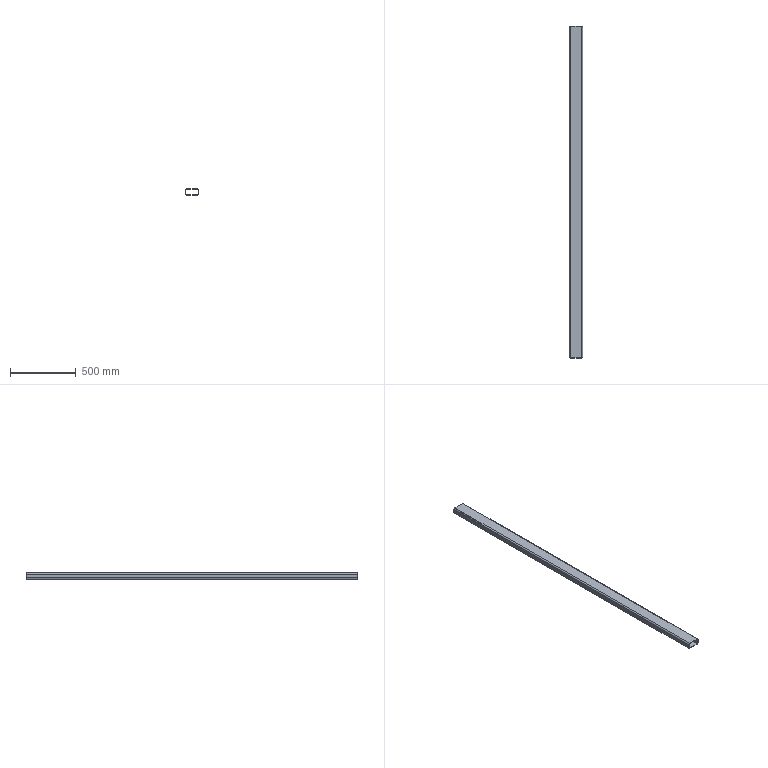Part | SolidWorks | features ExtruThin 1 | 1 solid | 18 faces | box 100 x 2530 x 50 mm | volume 2735087 mm3 | plane 10 | cylinder 8 | commonest cylinder face diameters 12 x4 20 x4
STEP:
#1=CARTESIAN_POINT('',(50.,1265.,-15.));
#2=VERTEX_POINT('',#1);
#3=CARTESIAN_POINT('',(40.,1265.,-25.));
#4=VERTEX_POINT('',#3);
#5=CARTESIAN_POINT('',(40.,1265.,-15.));
#6=DIRECTION('',(0.,1.,0.));
#7=DIRECTION('',(0.,0.,-1.));
#8=AXIS2_PLACEMENT_3D('',#5,#6,#7);
#9=CIRCLE('',#8,10.);
#10=EDGE_CURVE('',#2,#4,#9,.T.);
#11=ORIENTED_EDGE('',*,*,#10,.T.);
#12=CARTESIAN_POINT('',(-40.,1265.,-25.));
#13=VERTEX_POINT('',#12);
#14=CARTESIAN_POINT('',(-40.,1265.,-25.));
#15=DIRECTION('',(-1.,0.,0.));
#16=VECTOR('',#15,1000.);
#17=LINE('',#14,#16);
#18=EDGE_CURVE('',#4,#13,#17,.T.);
#19=ORIENTED_EDGE('',*,*,#18,.T.);
#20=CARTESIAN_POINT('',(-50.,1265.,-15.));
#21=VERTEX_POINT('',#20);
#22=CARTESIAN_POINT('',(-40.,1265.,-15.));
#23=DIRECTION('',(0.,1.,0.));
#24=DIRECTION('',(0.,0.,1.));
#25=AXIS2_PLACEMENT_3D('',#22,#23,#24);
#26=CIRCLE('',#25,10.);
#27=EDGE_CURVE('',#13,#21,#26,.T.);
#28=ORIENTED_EDGE('',*,*,#27,.T.);
#29=CARTESIAN_POINT('',(-50.,1265.,15.));
#30=VERTEX_POINT('',#29);
#31=CARTESIAN_POINT('',(-50.,1265.,-15.));
#32=DIRECTION('',(0.,0.,1.));
#33=VECTOR('',#32,1000.);
#34=LINE('',#31,#33);
#35=EDGE_CURVE('',#21,#30,#34,.T.);
#36=ORIENTED_EDGE('',*,*,#35,.T.);
#37=CARTESIAN_POINT('',(-40.,1265.,25.));
#38=VERTEX_POINT('',#37);
#39=CARTESIAN_POINT('',(-40.,1265.,15.));
#40=DIRECTION('',(0.,1.,0.));
#41=DIRECTION('',(0.,0.,1.));
#42=AXIS2_PLACEMENT_3D('',#39,#40,#41);
#43=CIRCLE('',#42,10.);
#44=EDGE_CURVE('',#30,#38,#43,.T.);
#45=ORIENTED_EDGE('',*,*,#44,.T.);
#46=CARTESIAN_POINT('',(40.,1265.,25.));
#47=VERTEX_POINT('',#46);
#48=CARTESIAN_POINT('',(-40.,1265.,25.));
#49=DIRECTION('',(1.,0.,0.));
#50=VECTOR('',#49,1000.);
#51=LINE('',#48,#50);
#52=EDGE_CURVE('',#38,#47,#51,.T.);
#53=ORIENTED_EDGE('',*,*,#52,.T.);
#54=CARTESIAN_POINT('',(50.,1265.,15.));
#55=VERTEX_POINT('',#54);
#56=CARTESIAN_POINT('',(40.,1265.,15.));
#57=DIRECTION('',(0.,1.,0.));
#58=DIRECTION('',(0.,0.,1.));
#59=AXIS2_PLACEMENT_3D('',#56,#57,#58);
#60=CIRCLE('',#59,10.);
#61=EDGE_CURVE('',#47,#55,#60,.T.);
#62=ORIENTED_EDGE('',*,*,#61,.T.);
#63=CARTESIAN_POINT('',(50.,1265.,-15.));
#64=DIRECTION('',(0.,0.,-1.));
#65=VECTOR('',#64,1000.);
#66=LINE('',#63,#65);
#67=EDGE_CURVE('',#55,#2,#66,.T.);
#68=ORIENTED_EDGE('',*,*,#67,.T.);
#69=EDGE_LOOP('',(#11,#19,#28,#36,#45,#53,#62,#68));
#70=FACE_OUTER_BOUND('',#69,.T.);
#71=CARTESIAN_POINT('',(40.,1265.,-21.));
#72=VERTEX_POINT('',#71);
#73=CARTESIAN_POINT('',(-40.,1265.,-21.));
#74=VERTEX_POINT('',#73);
#75=CARTESIAN_POINT('',(40.,1265.,-21.));
#76=DIRECTION('',(-1.,0.,0.));
#77=VECTOR('',#76,1000.);
#78=LINE('',#75,#77);
#79=EDGE_CURVE('',#72,#74,#78,.T.);
#80=ORIENTED_EDGE('',*,*,#79,.F.);
#81=CARTESIAN_POINT('',(46.,1265.,-15.));
#82=VERTEX_POINT('',#81);
#83=CARTESIAN_POINT('',(40.,1265.,-15.));
#84=DIRECTION('',(0.,1.,0.));
#85=DIRECTION('',(-1.,0.,0.));
#86=AXIS2_PLACEMENT_3D('',#83,#84,#85);
#87=CIRCLE('',#86,6.);
#88=EDGE_CURVE('',#82,#72,#87,.T.);
#89=ORIENTED_EDGE('',*,*,#88,.F.);
#90=CARTESIAN_POINT('',(46.,1265.,15.));
#91=VERTEX_POINT('',#90);
#92=CARTESIAN_POINT('',(46.,1265.,-15.));
#93=DIRECTION('',(0.,0.,-1.));
#94=VECTOR('',#93,1000.);
#95=LINE('',#92,#94);
#96=EDGE_CURVE('',#91,#82,#95,.T.);
#97=ORIENTED_EDGE('',*,*,#96,.F.);
#98=CARTESIAN_POINT('',(40.,1265.,21.));
#99=VERTEX_POINT('',#98);
#100=CARTESIAN_POINT('',(40.,1265.,15.));
#101=DIRECTION('',(0.,1.,0.));
#102=DIRECTION('',(-1.,0.,0.));
#103=AXIS2_PLACEMENT_3D('',#100,#101,#102);
#104=CIRCLE('',#103,6.);
#105=EDGE_CURVE('',#99,#91,#104,.T.);
#106=ORIENTED_EDGE('',*,*,#105,.F.);
#107=CARTESIAN_POINT('',(-40.,1265.,21.));
#108=VERTEX_POINT('',#107);
#109=CARTESIAN_POINT('',(40.,1265.,21.));
#110=DIRECTION('',(1.,0.,0.));
#111=VECTOR('',#110,1000.);
#112=LINE('',#109,#111);
#113=EDGE_CURVE('',#108,#99,#112,.T.);
#114=ORIENTED_EDGE('',*,*,#113,.F.);
#115=CARTESIAN_POINT('',(-46.,1265.,15.));
#116=VERTEX_POINT('',#115);
#117=CARTESIAN_POINT('',(-40.,1265.,15.));
#118=DIRECTION('',(0.,1.,0.));
#119=DIRECTION('',(-1.,0.,0.));
#120=AXIS2_PLACEMENT_3D('',#117,#118,#119);
#121=CIRCLE('',#120,6.);
#122=EDGE_CURVE('',#116,#108,#121,.T.);
#123=ORIENTED_EDGE('',*,*,#122,.F.);
#124=CARTESIAN_POINT('',(-46.,1265.,-15.));
#125=VERTEX_POINT('',#124);
#126=CARTESIAN_POINT('',(-46.,1265.,-15.));
#127=DIRECTION('',(0.,0.,1.));
#128=VECTOR('',#127,1000.);
#129=LINE('',#126,#128);
#130=EDGE_CURVE('',#125,#116,#129,.T.);
#131=ORIENTED_EDGE('',*,*,#130,.F.);
#132=CARTESIAN_POINT('',(-40.,1265.,-15.));
#133=DIRECTION('',(0.,1.,0.));
#134=DIRECTION('',(-1.,0.,0.));
#135=AXIS2_PLACEMENT_3D('',#132,#133,#134);
#136=CIRCLE('',#135,6.);
#137=EDGE_CURVE('',#74,#125,#136,.T.);
#138=ORIENTED_EDGE('',*,*,#137,.F.);
#139=EDGE_LOOP('',(#80,#89,#97,#106,#114,#123,#131,#138));
#140=FACE_BOUND('',#139,.T.);
#141=CARTESIAN_POINT('',(40.,1265.,-15.));
#142=DIRECTION('',(0.,1.,0.));
#143=DIRECTION('',(0.,0.,1.));
#144=AXIS2_PLACEMENT_3D('',#141,#142,#143);
#145=PLANE('',#144);
#146=ADVANCED_FACE('',(#70,#140),#145,.T.);
#147=CARTESIAN_POINT('',(50.,-1265.,-15.));
#148=VERTEX_POINT('',#147);
#149=CARTESIAN_POINT('',(40.,-1265.,-25.));
#150=VERTEX_POINT('',#149);
#151=CARTESIAN_POINT('',(40.,-1265.,-15.));
#152=DIRECTION('',(0.,1.,0.));
#153=DIRECTION('',(0.,0.,-1.));
#154=AXIS2_PLACEMENT_3D('',#151,#152,#153);
#155=CIRCLE('',#154,10.);
#156=EDGE_CURVE('',#148,#150,#155,.T.);
#157=ORIENTED_EDGE('',*,*,#156,.F.);
#158=CARTESIAN_POINT('',(50.,-1265.,15.));
#159=VERTEX_POINT('',#158);
#160=CARTESIAN_POINT('',(50.,-1265.,-15.));
#161=DIRECTION('',(0.,0.,-1.));
#162=VECTOR('',#161,1000.);
#163=LINE('',#160,#162);
#164=EDGE_CURVE('',#159,#148,#163,.T.);
#165=ORIENTED_EDGE('',*,*,#164,.F.);
#166=CARTESIAN_POINT('',(40.,-1265.,25.));
#167=VERTEX_POINT('',#166);
#168=CARTESIAN_POINT('',(40.,-1265.,15.));
#169=DIRECTION('',(0.,1.,0.));
#170=DIRECTION('',(0.,0.,1.));
#171=AXIS2_PLACEMENT_3D('',#168,#169,#170);
#172=CIRCLE('',#171,10.);
#173=EDGE_CURVE('',#167,#159,#172,.T.);
#174=ORIENTED_EDGE('',*,*,#173,.F.);
#175=CARTESIAN_POINT('',(-40.,-1265.,25.));
#176=VERTEX_POINT('',#175);
#177=CARTESIAN_POINT('',(-40.,-1265.,25.));
#178=DIRECTION('',(1.,0.,0.));
#179=VECTOR('',#178,1000.);
#180=LINE('',#177,#179);
#181=EDGE_CURVE('',#176,#167,#180,.T.);
#182=ORIENTED_EDGE('',*,*,#181,.F.);
#183=CARTESIAN_POINT('',(-50.,-1265.,15.));
#184=VERTEX_POINT('',#183);
#185=CARTESIAN_POINT('',(-40.,-1265.,15.));
#186=DIRECTION('',(0.,1.,0.));
#187=DIRECTION('',(0.,0.,1.));
#188=AXIS2_PLACEMENT_3D('',#185,#186,#187);
#189=CIRCLE('',#188,10.);
#190=EDGE_CURVE('',#184,#176,#189,.T.);
#191=ORIENTED_EDGE('',*,*,#190,.F.);
#192=CARTESIAN_POINT('',(-50.,-1265.,-15.));
#193=VERTEX_POINT('',#192);
#194=CARTESIAN_POINT('',(-50.,-1265.,-15.));
#195=DIRECTION('',(0.,0.,1.));
#196=VECTOR('',#195,1000.);
#197=LINE('',#194,#196);
#198=EDGE_CURVE('',#193,#184,#197,.T.);
#199=ORIENTED_EDGE('',*,*,#198,.F.);
#200=CARTESIAN_POINT('',(-40.,-1265.,-25.));
#201=VERTEX_POINT('',#200);
#202=CARTESIAN_POINT('',(-40.,-1265.,-15.));
#203=DIRECTION('',(0.,1.,0.));
#204=DIRECTION('',(0.,0.,1.));
#205=AXIS2_PLACEMENT_3D('',#202,#203,#204);
#206=CIRCLE('',#205,10.);
#207=EDGE_CURVE('',#201,#193,#206,.T.);
#208=ORIENTED_EDGE('',*,*,#207,.F.);
#209=CARTESIAN_POINT('',(-40.,-1265.,-25.));
#210=DIRECTION('',(-1.,0.,0.));
#211=VECTOR('',#210,1000.);
#212=LINE('',#209,#211);
#213=EDGE_CURVE('',#150,#201,#212,.T.);
#214=ORIENTED_EDGE('',*,*,#213,.F.);
#215=EDGE_LOOP('',(#157,#165,#174,#182,#191,#199,#208,#214));
#216=FACE_OUTER_BOUND('',#215,.T.);
#217=CARTESIAN_POINT('',(46.,-1265.,-15.));
#218=VERTEX_POINT('',#217);
#219=CARTESIAN_POINT('',(40.,-1265.,-21.));
#220=VERTEX_POINT('',#219);
#221=CARTESIAN_POINT('',(40.,-1265.,-15.));
#222=DIRECTION('',(0.,1.,0.));
#223=DIRECTION('',(-1.,0.,0.));
#224=AXIS2_PLACEMENT_3D('',#221,#222,#223);
#225=CIRCLE('',#224,6.);
#226=EDGE_CURVE('',#218,#220,#225,.T.);
#227=ORIENTED_EDGE('',*,*,#226,.T.);
#228=CARTESIAN_POINT('',(-40.,-1265.,-21.));
#229=VERTEX_POINT('',#228);
#230=CARTESIAN_POINT('',(40.,-1265.,-21.));
#231=DIRECTION('',(-1.,0.,0.));
#232=VECTOR('',#231,1000.);
#233=LINE('',#230,#232);
#234=EDGE_CURVE('',#220,#229,#233,.T.);
#235=ORIENTED_EDGE('',*,*,#234,.T.);
#236=CARTESIAN_POINT('',(-46.,-1265.,-15.));
#237=VERTEX_POINT('',#236);
#238=CARTESIAN_POINT('',(-40.,-1265.,-15.));
#239=DIRECTION('',(0.,1.,0.));
#240=DIRECTION('',(-1.,0.,0.));
#241=AXIS2_PLACEMENT_3D('',#238,#239,#240);
#242=CIRCLE('',#241,6.);
#243=EDGE_CURVE('',#229,#237,#242,.T.);
#244=ORIENTED_EDGE('',*,*,#243,.T.);
#245=CARTESIAN_POINT('',(-46.,-1265.,15.));
#246=VERTEX_POINT('',#245);
#247=CARTESIAN_POINT('',(-46.,-1265.,-15.));
#248=DIRECTION('',(0.,0.,1.));
#249=VECTOR('',#248,1000.);
#250=LINE('',#247,#249);
#251=EDGE_CURVE('',#237,#246,#250,.T.);
#252=ORIENTED_EDGE('',*,*,#251,.T.);
#253=CARTESIAN_POINT('',(-40.,-1265.,21.));
#254=VERTEX_POINT('',#253);
#255=CARTESIAN_POINT('',(-40.,-1265.,15.));
#256=DIRECTION('',(0.,1.,0.));
#257=DIRECTION('',(-1.,0.,0.));
#258=AXIS2_PLACEMENT_3D('',#255,#256,#257);
#259=CIRCLE('',#258,6.);
#260=EDGE_CURVE('',#246,#254,#259,.T.);
#261=ORIENTED_EDGE('',*,*,#260,.T.);
#262=CARTESIAN_POINT('',(40.,-1265.,21.));
#263=VERTEX_POINT('',#262);
#264=CARTESIAN_POINT('',(40.,-1265.,21.));
#265=DIRECTION('',(1.,0.,0.));
#266=VECTOR('',#265,1000.);
#267=LINE('',#264,#266);
#268=EDGE_CURVE('',#254,#263,#267,.T.);
#269=ORIENTED_EDGE('',*,*,#268,.T.);
#270=CARTESIAN_POINT('',(46.,-1265.,15.));
#271=VERTEX_POINT('',#270);
#272=CARTESIAN_POINT('',(40.,-1265.,15.));
#273=DIRECTION('',(0.,1.,0.));
#274=DIRECTION('',(-1.,0.,0.));
#275=AXIS2_PLACEMENT_3D('',#272,#273,#274);
#276=CIRCLE('',#275,6.);
#277=EDGE_CURVE('',#263,#271,#276,.T.);
#278=ORIENTED_EDGE('',*,*,#277,.T.);
#279=CARTESIAN_POINT('',(46.,-1265.,-15.));
#280=DIRECTION('',(0.,0.,-1.));
#281=VECTOR('',#280,1000.);
#282=LINE('',#279,#281);
#283=EDGE_CURVE('',#271,#218,#282,.T.);
#284=ORIENTED_EDGE('',*,*,#283,.T.);
#285=EDGE_LOOP('',(#227,#235,#244,#252,#261,#269,#278,#284));
#286=FACE_BOUND('',#285,.T.);
#287=CARTESIAN_POINT('',(40.,-1265.,-15.));
#288=DIRECTION('',(0.,1.,0.));
#289=DIRECTION('',(0.,0.,1.));
#290=AXIS2_PLACEMENT_3D('',#287,#288,#289);
#291=PLANE('',#290);
#292=ADVANCED_FACE('',(#216,#286),#291,.F.);
#293=ORIENTED_EDGE('',*,*,#156,.T.);
#294=CARTESIAN_POINT('',(40.,1265.,-25.));
#295=DIRECTION('',(0.,-1.,0.));
#296=VECTOR('',#295,1000.);
#297=LINE('',#294,#296);
#298=EDGE_CURVE('',#4,#150,#297,.T.);
#299=ORIENTED_EDGE('',*,*,#298,.F.);
#300=ORIENTED_EDGE('',*,*,#10,.F.);
#301=CARTESIAN_POINT('',(50.,1265.,-15.));
#302=DIRECTION('',(0.,-1.,0.));
#303=VECTOR('',#302,1000.);
#304=LINE('',#301,#303);
#305=EDGE_CURVE('',#2,#148,#304,.T.);
#306=ORIENTED_EDGE('',*,*,#305,.T.);
#307=EDGE_LOOP('',(#293,#299,#300,#306));
#308=FACE_OUTER_BOUND('',#307,.T.);
#309=CARTESIAN_POINT('',(40.,1265.,-15.));
#310=DIRECTION('',(0.,-1.,0.));
#311=DIRECTION('',(0.,0.,-1.));
#312=AXIS2_PLACEMENT_3D('',#309,#310,#311);
#313=CYLINDRICAL_SURFACE('',#312,10.);
#314=ADVANCED_FACE('',(#308),#313,.T.);
#315=ORIENTED_EDGE('',*,*,#213,.T.);
#316=CARTESIAN_POINT('',(-40.,1265.,-25.));
#317=DIRECTION('',(0.,-1.,0.));
#318=VECTOR('',#317,1000.);
#319=LINE('',#316,#318);
#320=EDGE_CURVE('',#13,#201,#319,.T.);
#321=ORIENTED_EDGE('',*,*,#320,.F.);
#322=ORIENTED_EDGE('',*,*,#18,.F.);
#323=ORIENTED_EDGE('',*,*,#298,.T.);
#324=EDGE_LOOP('',(#315,#321,#322,#323));
#325=FACE_OUTER_BOUND('',#324,.T.);
#326=CARTESIAN_POINT('',(-40.,1265.,-25.));
#327=DIRECTION('',(0.,0.,1.));
#328=DIRECTION('',(1.,0.,0.));
#329=AXIS2_PLACEMENT_3D('',#326,#327,#328);
#330=PLANE('',#329);
#331=ADVANCED_FACE('',(#325),#330,.F.);
#332=ORIENTED_EDGE('',*,*,#207,.T.);
#333=CARTESIAN_POINT('',(-50.,1265.,-15.));
#334=DIRECTION('',(0.,-1.,0.));
#335=VECTOR('',#334,1000.);
#336=LINE('',#333,#335);
#337=EDGE_CURVE('',#21,#193,#336,.T.);
#338=ORIENTED_EDGE('',*,*,#337,.F.);
#339=ORIENTED_EDGE('',*,*,#27,.F.);
#340=ORIENTED_EDGE('',*,*,#320,.T.);
#341=EDGE_LOOP('',(#332,#338,#339,#340));
#342=FACE_OUTER_BOUND('',#341,.T.);
#343=CARTESIAN_POINT('',(-40.,1265.,-15.));
#344=DIRECTION('',(0.,-1.,0.));
#345=DIRECTION('',(0.,0.,-1.));
#346=AXIS2_PLACEMENT_3D('',#343,#344,#345);
#347=CYLINDRICAL_SURFACE('',#346,10.);
#348=ADVANCED_FACE('',(#342),#347,.T.);
#349=ORIENTED_EDGE('',*,*,#198,.T.);
#350=CARTESIAN_POINT('',(-50.,1265.,15.));
#351=DIRECTION('',(0.,-1.,0.));
#352=VECTOR('',#351,1000.);
#353=LINE('',#350,#352);
#354=EDGE_CURVE('',#30,#184,#353,.T.);
#355=ORIENTED_EDGE('',*,*,#354,.F.);
#356=ORIENTED_EDGE('',*,*,#35,.F.);
#357=ORIENTED_EDGE('',*,*,#337,.T.);
#358=EDGE_LOOP('',(#349,#355,#356,#357));
#359=FACE_OUTER_BOUND('',#358,.T.);
#360=CARTESIAN_POINT('',(-50.,1265.,-15.));
#361=DIRECTION('',(1.,0.,0.));
#362=DIRECTION('',(0.,0.,-1.));
#363=AXIS2_PLACEMENT_3D('',#360,#361,#362);
#364=PLANE('',#363);
#365=ADVANCED_FACE('',(#359),#364,.F.);
#366=ORIENTED_EDGE('',*,*,#190,.T.);
#367=CARTESIAN_POINT('',(-40.,1265.,25.));
#368=DIRECTION('',(0.,-1.,0.));
#369=VECTOR('',#368,1000.);
#370=LINE('',#367,#369);
#371=EDGE_CURVE('',#38,#176,#370,.T.);
#372=ORIENTED_EDGE('',*,*,#371,.F.);
#373=ORIENTED_EDGE('',*,*,#44,.F.);
#374=ORIENTED_EDGE('',*,*,#354,.T.);
#375=EDGE_LOOP('',(#366,#372,#373,#374));
#376=FACE_OUTER_BOUND('',#375,.T.);
#377=CARTESIAN_POINT('',(-40.,1265.,15.));
#378=DIRECTION('',(0.,-1.,0.));
#379=DIRECTION('',(0.,0.,-1.));
#380=AXIS2_PLACEMENT_3D('',#377,#378,#379);
#381=CYLINDRICAL_SURFACE('',#380,10.);
#382=ADVANCED_FACE('',(#376),#381,.T.);
#383=ORIENTED_EDGE('',*,*,#181,.T.);
#384=CARTESIAN_POINT('',(40.,1265.,25.));
#385=DIRECTION('',(0.,-1.,0.));
#386=VECTOR('',#385,1000.);
#387=LINE('',#384,#386);
#388=EDGE_CURVE('',#47,#167,#387,.T.);
#389=ORIENTED_EDGE('',*,*,#388,.F.);
#390=ORIENTED_EDGE('',*,*,#52,.F.);
#391=ORIENTED_EDGE('',*,*,#371,.T.);
#392=EDGE_LOOP('',(#383,#389,#390,#391));
#393=FACE_OUTER_BOUND('',#392,.T.);
#394=CARTESIAN_POINT('',(-40.,1265.,25.));
#395=DIRECTION('',(0.,0.,-1.));
#396=DIRECTION('',(-1.,0.,0.));
#397=AXIS2_PLACEMENT_3D('',#394,#395,#396);
#398=PLANE('',#397);
#399=ADVANCED_FACE('',(#393),#398,.F.);
#400=ORIENTED_EDGE('',*,*,#173,.T.);
#401=CARTESIAN_POINT('',(50.,1265.,15.));
#402=DIRECTION('',(0.,-1.,0.));
#403=VECTOR('',#402,1000.);
#404=LINE('',#401,#403);
#405=EDGE_CURVE('',#55,#159,#404,.T.);
#406=ORIENTED_EDGE('',*,*,#405,.F.);
#407=ORIENTED_EDGE('',*,*,#61,.F.);
#408=ORIENTED_EDGE('',*,*,#388,.T.);
#409=EDGE_LOOP('',(#400,#406,#407,#408));
#410=FACE_OUTER_BOUND('',#409,.T.);
#411=CARTESIAN_POINT('',(40.,1265.,15.));
#412=DIRECTION('',(0.,-1.,0.));
#413=DIRECTION('',(0.,0.,-1.));
#414=AXIS2_PLACEMENT_3D('',#411,#412,#413);
#415=CYLINDRICAL_SURFACE('',#414,10.);
#416=ADVANCED_FACE('',(#410),#415,.T.);
#417=ORIENTED_EDGE('',*,*,#164,.T.);
#418=ORIENTED_EDGE('',*,*,#305,.F.);
#419=ORIENTED_EDGE('',*,*,#67,.F.);
#420=ORIENTED_EDGE('',*,*,#405,.T.);
#421=EDGE_LOOP('',(#417,#418,#419,#420));
#422=FACE_OUTER_BOUND('',#421,.T.);
#423=CARTESIAN_POINT('',(50.,1265.,-15.));
#424=DIRECTION('',(-1.,0.,0.));
#425=DIRECTION('',(0.,0.,1.));
#426=AXIS2_PLACEMENT_3D('',#423,#424,#425);
#427=PLANE('',#426);
#428=ADVANCED_FACE('',(#422),#427,.F.);
#429=ORIENTED_EDGE('',*,*,#226,.F.);
#430=CARTESIAN_POINT('',(46.,1265.,-15.));
#431=DIRECTION('',(0.,-1.,0.));
#432=VECTOR('',#431,1000.);
#433=LINE('',#430,#432);
#434=EDGE_CURVE('',#82,#218,#433,.T.);
#435=ORIENTED_EDGE('',*,*,#434,.F.);
#436=ORIENTED_EDGE('',*,*,#88,.T.);
#437=CARTESIAN_POINT('',(40.,1265.,-21.));
#438=DIRECTION('',(0.,-1.,0.));
#439=VECTOR('',#438,1000.);
#440=LINE('',#437,#439);
#441=EDGE_CURVE('',#72,#220,#440,.T.);
#442=ORIENTED_EDGE('',*,*,#441,.T.);
#443=EDGE_LOOP('',(#429,#435,#436,#442));
#444=FACE_OUTER_BOUND('',#443,.T.);
#445=CARTESIAN_POINT('',(40.,1265.,-15.));
#446=DIRECTION('',(0.,-1.,0.));
#447=DIRECTION('',(0.,0.,-1.));
#448=AXIS2_PLACEMENT_3D('',#445,#446,#447);
#449=CYLINDRICAL_SURFACE('',#448,6.);
#450=ADVANCED_FACE('',(#444),#449,.F.);
#451=ORIENTED_EDGE('',*,*,#234,.F.);
#452=ORIENTED_EDGE('',*,*,#441,.F.);
#453=ORIENTED_EDGE('',*,*,#79,.T.);
#454=CARTESIAN_POINT('',(-40.,1265.,-21.));
#455=DIRECTION('',(0.,-1.,0.));
#456=VECTOR('',#455,1000.);
#457=LINE('',#454,#456);
#458=EDGE_CURVE('',#74,#229,#457,.T.);
#459=ORIENTED_EDGE('',*,*,#458,.T.);
#460=EDGE_LOOP('',(#451,#452,#453,#459));
#461=FACE_OUTER_BOUND('',#460,.T.);
#462=CARTESIAN_POINT('',(40.,1265.,-21.));
#463=DIRECTION('',(0.,0.,1.));
#464=DIRECTION('',(1.,0.,0.));
#465=AXIS2_PLACEMENT_3D('',#462,#463,#464);
#466=PLANE('',#465);
#467=ADVANCED_FACE('',(#461),#466,.T.);
#468=ORIENTED_EDGE('',*,*,#243,.F.);
#469=ORIENTED_EDGE('',*,*,#458,.F.);
#470=ORIENTED_EDGE('',*,*,#137,.T.);
#471=CARTESIAN_POINT('',(-46.,1265.,-15.));
#472=DIRECTION('',(0.,-1.,0.));
#473=VECTOR('',#472,1000.);
#474=LINE('',#471,#473);
#475=EDGE_CURVE('',#125,#237,#474,.T.);
#476=ORIENTED_EDGE('',*,*,#475,.T.);
#477=EDGE_LOOP('',(#468,#469,#470,#476));
#478=FACE_OUTER_BOUND('',#477,.T.);
#479=CARTESIAN_POINT('',(-40.,1265.,-15.));
#480=DIRECTION('',(0.,-1.,0.));
#481=DIRECTION('',(0.,0.,-1.));
#482=AXIS2_PLACEMENT_3D('',#479,#480,#481);
#483=CYLINDRICAL_SURFACE('',#482,6.);
#484=ADVANCED_FACE('',(#478),#483,.F.);
#485=ORIENTED_EDGE('',*,*,#251,.F.);
#486=ORIENTED_EDGE('',*,*,#475,.F.);
#487=ORIENTED_EDGE('',*,*,#130,.T.);
#488=CARTESIAN_POINT('',(-46.,1265.,15.));
#489=DIRECTION('',(0.,-1.,0.));
#490=VECTOR('',#489,1000.);
#491=LINE('',#488,#490);
#492=EDGE_CURVE('',#116,#246,#491,.T.);
#493=ORIENTED_EDGE('',*,*,#492,.T.);
#494=EDGE_LOOP('',(#485,#486,#487,#493));
#495=FACE_OUTER_BOUND('',#494,.T.);
#496=CARTESIAN_POINT('',(-46.,1265.,-15.));
#497=DIRECTION('',(1.,0.,0.));
#498=DIRECTION('',(0.,0.,-1.));
#499=AXIS2_PLACEMENT_3D('',#496,#497,#498);
#500=PLANE('',#499);
#501=ADVANCED_FACE('',(#495),#500,.T.);
#502=ORIENTED_EDGE('',*,*,#260,.F.);
#503=ORIENTED_EDGE('',*,*,#492,.F.);
#504=ORIENTED_EDGE('',*,*,#122,.T.);
#505=CARTESIAN_POINT('',(-40.,1265.,21.));
#506=DIRECTION('',(0.,-1.,0.));
#507=VECTOR('',#506,1000.);
#508=LINE('',#505,#507);
#509=EDGE_CURVE('',#108,#254,#508,.T.);
#510=ORIENTED_EDGE('',*,*,#509,.T.);
#511=EDGE_LOOP('',(#502,#503,#504,#510));
#512=FACE_OUTER_BOUND('',#511,.T.);
#513=CARTESIAN_POINT('',(-40.,1265.,15.));
#514=DIRECTION('',(0.,-1.,0.));
#515=DIRECTION('',(0.,0.,-1.));
#516=AXIS2_PLACEMENT_3D('',#513,#514,#515);
#517=CYLINDRICAL_SURFACE('',#516,6.);
#518=ADVANCED_FACE('',(#512),#517,.F.);
#519=ORIENTED_EDGE('',*,*,#268,.F.);
#520=ORIENTED_EDGE('',*,*,#509,.F.);
#521=ORIENTED_EDGE('',*,*,#113,.T.);
#522=CARTESIAN_POINT('',(40.,1265.,21.));
#523=DIRECTION('',(0.,-1.,0.));
#524=VECTOR('',#523,1000.);
#525=LINE('',#522,#524);
#526=EDGE_CURVE('',#99,#263,#525,.T.);
#527=ORIENTED_EDGE('',*,*,#526,.T.);
#528=EDGE_LOOP('',(#519,#520,#521,#527));
#529=FACE_OUTER_BOUND('',#528,.T.);
#530=CARTESIAN_POINT('',(40.,1265.,21.));
#531=DIRECTION('',(0.,0.,-1.));
#532=DIRECTION('',(-1.,0.,0.));
#533=AXIS2_PLACEMENT_3D('',#530,#531,#532);
#534=PLANE('',#533);
#535=ADVANCED_FACE('',(#529),#534,.T.);
#536=ORIENTED_EDGE('',*,*,#277,.F.);
#537=ORIENTED_EDGE('',*,*,#526,.F.);
#538=ORIENTED_EDGE('',*,*,#105,.T.);
#539=CARTESIAN_POINT('',(46.,1265.,15.));
#540=DIRECTION('',(0.,-1.,0.));
#541=VECTOR('',#540,1000.);
#542=LINE('',#539,#541);
#543=EDGE_CURVE('',#91,#271,#542,.T.);
#544=ORIENTED_EDGE('',*,*,#543,.T.);
#545=EDGE_LOOP('',(#536,#537,#538,#544));
#546=FACE_OUTER_BOUND('',#545,.T.);
#547=CARTESIAN_POINT('',(40.,1265.,15.));
#548=DIRECTION('',(0.,-1.,0.));
#549=DIRECTION('',(0.,0.,-1.));
#550=AXIS2_PLACEMENT_3D('',#547,#548,#549);
#551=CYLINDRICAL_SURFACE('',#550,6.);
#552=ADVANCED_FACE('',(#546),#551,.F.);
#553=ORIENTED_EDGE('',*,*,#283,.F.);
#554=ORIENTED_EDGE('',*,*,#543,.F.);
#555=ORIENTED_EDGE('',*,*,#96,.T.);
#556=ORIENTED_EDGE('',*,*,#434,.T.);
#557=EDGE_LOOP('',(#553,#554,#555,#556));
#558=FACE_OUTER_BOUND('',#557,.T.);
#559=CARTESIAN_POINT('',(46.,1265.,-15.));
#560=DIRECTION('',(-1.,0.,0.));
#561=DIRECTION('',(0.,0.,1.));
#562=AXIS2_PLACEMENT_3D('',#559,#560,#561);
#563=PLANE('',#562);
#564=ADVANCED_FACE('',(#558),#563,.T.);
#565=CLOSED_SHELL('',(#146,#292,#314,#331,#348,#365,#382,#399,#416,#428,#450,#467,#484,#501,#518,#535,#552,#564));
#566=MANIFOLD_SOLID_BREP('',#565);
#567=CARTESIAN_POINT('',(0.,0.,0.));
#568=DIRECTION('',(0.,0.,1.));
#569=DIRECTION('',(1.,0.,0.));
#570=AXIS2_PLACEMENT_3D('',#567,#568,#569);
#571=(LENGTH_UNIT()NAMED_UNIT(*)SI_UNIT(.MILLI.,.METRE.));
#572=UNCERTAINTY_MEASURE_WITH_UNIT(LENGTH_MEASURE(0.00001),#571,'','');
#573=(NAMED_UNIT(*)PLANE_ANGLE_UNIT()SI_UNIT($,.RADIAN.));
#574=(NAMED_UNIT(*)SI_UNIT($,.STERADIAN.)SOLID_ANGLE_UNIT());
#575=(GEOMETRIC_REPRESENTATION_CONTEXT(3)GLOBAL_UNCERTAINTY_ASSIGNED_CONTEXT((#572))GLOBAL_UNIT_ASSIGNED_CONTEXT((#571,#573,#574))REPRESENTATION_CONTEXT('',''));
#576=ADVANCED_BREP_SHAPE_REPRESENTATION('',(#566,#570),#575);